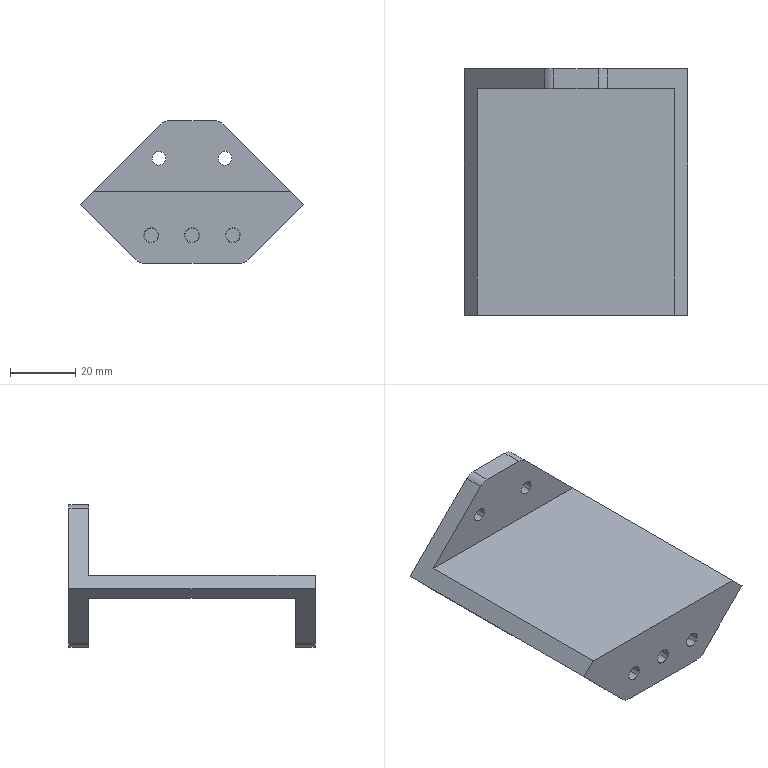Part | 1 solid | 42 faces | box 68.307 x 75.3 x 43.668 mm | volume 47119 mm3 | cylinder 20 | plane 16 | cone 6 | commonest cylinder face diameters 4.3 x6 8 x6 4 x4 4.2 x4
STEP:
#1=CARTESIAN_POINT('',(11.596,37.65,-13.01));
#2=VERTEX_POINT('',#1);
#3=CARTESIAN_POINT('',(8.626,37.65,-10.041));
#4=VERTEX_POINT('',#3);
#5=CARTESIAN_POINT('',(10.111,37.65,-11.525));
#6=DIRECTION('',(0.,-1.,0.));
#7=DIRECTION('',(-0.7071,0.,0.7071));
#8=AXIS2_PLACEMENT_3D('',#5,#6,#7);
#9=CIRCLE('',#8,2.1);
#10=EDGE_CURVE('',#2,#4,#9,.T.);
#11=ORIENTED_EDGE('',*,*,#10,.F.);
#12=CARTESIAN_POINT('',(11.596,31.65,-13.01));
#13=VERTEX_POINT('',#12);
#14=CARTESIAN_POINT('',(11.596,41.65,-13.01));
#15=DIRECTION('',(0.,-1.,0.));
#16=VECTOR('',#15,1000.);
#17=LINE('',#14,#16);
#18=EDGE_CURVE('',#13,#2,#17,.F.);
#19=ORIENTED_EDGE('',*,*,#18,.F.);
#20=CARTESIAN_POINT('',(8.626,31.65,-10.041));
#21=VERTEX_POINT('',#20);
#22=CARTESIAN_POINT('',(10.111,31.65,-11.525));
#23=DIRECTION('',(0.,-1.,0.));
#24=DIRECTION('',(-0.7071,0.,0.7071));
#25=AXIS2_PLACEMENT_3D('',#22,#23,#24);
#26=CIRCLE('',#25,2.1);
#27=EDGE_CURVE('',#13,#21,#26,.T.);
#28=ORIENTED_EDGE('',*,*,#27,.T.);
#29=CARTESIAN_POINT('',(8.626,41.65,-10.041));
#30=DIRECTION('',(0.,-1.,0.));
#31=VECTOR('',#30,1000.);
#32=LINE('',#29,#31);
#33=EDGE_CURVE('',#21,#4,#32,.F.);
#34=ORIENTED_EDGE('',*,*,#33,.T.);
#35=EDGE_LOOP('',(#11,#19,#28,#34));
#36=FACE_BOUND('',#35,.T.);
#37=CARTESIAN_POINT('',(10.111,41.65,-11.525));
#38=DIRECTION('',(0.,-1.,0.));
#39=DIRECTION('',(0.7071,0.,-0.7071));
#40=AXIS2_PLACEMENT_3D('',#37,#38,#39);
#41=CYLINDRICAL_SURFACE('',#40,2.1);
#42=ADVANCED_FACE('',(#36),#41,.F.);
#43=CARTESIAN_POINT('',(-8.626,37.65,-13.01));
#44=VERTEX_POINT('',#43);
#45=CARTESIAN_POINT('',(-11.596,37.65,-10.041));
#46=VERTEX_POINT('',#45);
#47=CARTESIAN_POINT('',(-10.111,37.65,-11.525));
#48=DIRECTION('',(0.,-1.,0.));
#49=DIRECTION('',(-0.7071,0.,0.7071));
#50=AXIS2_PLACEMENT_3D('',#47,#48,#49);
#51=CIRCLE('',#50,2.1);
#52=EDGE_CURVE('',#44,#46,#51,.T.);
#53=ORIENTED_EDGE('',*,*,#52,.F.);
#54=CARTESIAN_POINT('',(-8.626,31.65,-13.01));
#55=VERTEX_POINT('',#54);
#56=CARTESIAN_POINT('',(-8.626,41.65,-13.01));
#57=DIRECTION('',(0.,-1.,0.));
#58=VECTOR('',#57,1000.);
#59=LINE('',#56,#58);
#60=EDGE_CURVE('',#55,#44,#59,.F.);
#61=ORIENTED_EDGE('',*,*,#60,.F.);
#62=CARTESIAN_POINT('',(-11.596,31.65,-10.041));
#63=VERTEX_POINT('',#62);
#64=CARTESIAN_POINT('',(-10.111,31.65,-11.525));
#65=DIRECTION('',(0.,-1.,0.));
#66=DIRECTION('',(-0.7071,0.,0.7071));
#67=AXIS2_PLACEMENT_3D('',#64,#65,#66);
#68=CIRCLE('',#67,2.1);
#69=EDGE_CURVE('',#55,#63,#68,.T.);
#70=ORIENTED_EDGE('',*,*,#69,.T.);
#71=CARTESIAN_POINT('',(-11.596,41.65,-10.041));
#72=DIRECTION('',(0.,-1.,0.));
#73=VECTOR('',#72,1000.);
#74=LINE('',#71,#73);
#75=EDGE_CURVE('',#63,#46,#74,.F.);
#76=ORIENTED_EDGE('',*,*,#75,.T.);
#77=EDGE_LOOP('',(#53,#61,#70,#76));
#78=FACE_BOUND('',#77,.T.);
#79=CARTESIAN_POINT('',(-10.111,41.65,-11.525));
#80=DIRECTION('',(0.,-1.,0.));
#81=DIRECTION('',(0.7071,0.,-0.7071));
#82=AXIS2_PLACEMENT_3D('',#79,#80,#81);
#83=CYLINDRICAL_SURFACE('',#82,2.1);
#84=ADVANCED_FACE('',(#78),#83,.F.);
#85=CARTESIAN_POINT('',(3.536,33.65,-4.95));
#86=VERTEX_POINT('',#85);
#87=CARTESIAN_POINT('',(6.364,33.65,-7.778));
#88=VERTEX_POINT('',#87);
#89=CARTESIAN_POINT('',(4.95,33.65,-6.364));
#90=DIRECTION('',(0.,1.,0.));
#91=DIRECTION('',(0.7071,0.,-0.7071));
#92=AXIS2_PLACEMENT_3D('',#89,#90,#91);
#93=CIRCLE('',#92,2.);
#94=EDGE_CURVE('',#86,#88,#93,.T.);
#95=ORIENTED_EDGE('',*,*,#94,.F.);
#96=CARTESIAN_POINT('',(3.536,37.65,-4.95));
#97=VERTEX_POINT('',#96);
#98=CARTESIAN_POINT('',(3.536,33.65,-4.95));
#99=DIRECTION('',(0.,1.,0.));
#100=VECTOR('',#99,1000.);
#101=LINE('',#98,#100);
#102=EDGE_CURVE('',#97,#86,#101,.F.);
#103=ORIENTED_EDGE('',*,*,#102,.F.);
#104=CARTESIAN_POINT('',(6.364,37.65,-7.778));
#105=VERTEX_POINT('',#104);
#106=CARTESIAN_POINT('',(4.95,37.65,-6.364));
#107=DIRECTION('',(0.,1.,0.));
#108=DIRECTION('',(0.7071,0.,-0.7071));
#109=AXIS2_PLACEMENT_3D('',#106,#107,#108);
#110=CIRCLE('',#109,2.);
#111=EDGE_CURVE('',#97,#105,#110,.T.);
#112=ORIENTED_EDGE('',*,*,#111,.T.);
#113=CARTESIAN_POINT('',(6.364,33.65,-7.778));
#114=DIRECTION('',(0.,1.,0.));
#115=VECTOR('',#114,1000.);
#116=LINE('',#113,#115);
#117=EDGE_CURVE('',#105,#88,#116,.F.);
#118=ORIENTED_EDGE('',*,*,#117,.T.);
#119=EDGE_LOOP('',(#95,#103,#112,#118));
#120=FACE_BOUND('',#119,.T.);
#121=CARTESIAN_POINT('',(4.95,33.65,-6.364));
#122=DIRECTION('',(0.,1.,0.));
#123=DIRECTION('',(-0.7071,0.,0.7071));
#124=AXIS2_PLACEMENT_3D('',#121,#122,#123);
#125=CYLINDRICAL_SURFACE('',#124,2.);
#126=ADVANCED_FACE('',(#120),#125,.F.);
#127=CARTESIAN_POINT('',(-5.657,33.65,-14.142));
#128=VERTEX_POINT('',#127);
#129=CARTESIAN_POINT('',(-2.828,33.65,-16.971));
#130=VERTEX_POINT('',#129);
#131=CARTESIAN_POINT('',(-4.243,33.65,-15.556));
#132=DIRECTION('',(0.,1.,0.));
#133=DIRECTION('',(0.7071,0.,-0.7071));
#134=AXIS2_PLACEMENT_3D('',#131,#132,#133);
#135=CIRCLE('',#134,2.);
#136=EDGE_CURVE('',#128,#130,#135,.T.);
#137=ORIENTED_EDGE('',*,*,#136,.F.);
#138=CARTESIAN_POINT('',(-5.657,37.65,-14.142));
#139=VERTEX_POINT('',#138);
#140=CARTESIAN_POINT('',(-5.657,33.65,-14.142));
#141=DIRECTION('',(0.,1.,0.));
#142=VECTOR('',#141,1000.);
#143=LINE('',#140,#142);
#144=EDGE_CURVE('',#139,#128,#143,.F.);
#145=ORIENTED_EDGE('',*,*,#144,.F.);
#146=CARTESIAN_POINT('',(-2.828,37.65,-16.971));
#147=VERTEX_POINT('',#146);
#148=CARTESIAN_POINT('',(-4.243,37.65,-15.556));
#149=DIRECTION('',(0.,1.,0.));
#150=DIRECTION('',(0.7071,0.,-0.7071));
#151=AXIS2_PLACEMENT_3D('',#148,#149,#150);
#152=CIRCLE('',#151,2.);
#153=EDGE_CURVE('',#139,#147,#152,.T.);
#154=ORIENTED_EDGE('',*,*,#153,.T.);
#155=CARTESIAN_POINT('',(-2.828,33.65,-16.971));
#156=DIRECTION('',(0.,1.,0.));
#157=VECTOR('',#156,1000.);
#158=LINE('',#155,#157);
#159=EDGE_CURVE('',#147,#130,#158,.F.);
#160=ORIENTED_EDGE('',*,*,#159,.T.);
#161=EDGE_LOOP('',(#137,#145,#154,#160));
#162=FACE_BOUND('',#161,.T.);
#163=CARTESIAN_POINT('',(-4.243,33.65,-15.556));
#164=DIRECTION('',(0.,1.,0.));
#165=DIRECTION('',(-0.7071,0.,0.7071));
#166=AXIS2_PLACEMENT_3D('',#163,#164,#165);
#167=CYLINDRICAL_SURFACE('',#166,2.);
#168=ADVANCED_FACE('',(#162),#167,.F.);
#169=CARTESIAN_POINT('',(14.02,-37.525,-36.593));
#170=VERTEX_POINT('',#169);
#171=CARTESIAN_POINT('',(10.98,-37.525,-33.552));
#172=VERTEX_POINT('',#171);
#173=CARTESIAN_POINT('',(12.5,-37.525,-35.072));
#174=DIRECTION('',(0.,-1.,0.));
#175=DIRECTION('',(-0.7071,0.,0.7071));
#176=AXIS2_PLACEMENT_3D('',#173,#174,#175);
#177=CIRCLE('',#176,2.15);
#178=EDGE_CURVE('',#170,#172,#177,.T.);
#179=ORIENTED_EDGE('',*,*,#178,.F.);
#180=CARTESIAN_POINT('',(14.109,-37.65,-36.681));
#181=VERTEX_POINT('',#180);
#182=CARTESIAN_POINT('',(14.109,-37.65,-36.681));
#183=DIRECTION('',(0.5,-0.7071,-0.5));
#184=VECTOR('',#183,1000.);
#185=LINE('',#182,#184);
#186=EDGE_CURVE('',#181,#170,#185,.F.);
#187=ORIENTED_EDGE('',*,*,#186,.F.);
#188=CARTESIAN_POINT('',(10.891,-37.65,-33.464));
#189=VERTEX_POINT('',#188);
#190=CARTESIAN_POINT('',(12.5,-37.65,-35.072));
#191=DIRECTION('',(0.,-1.,0.));
#192=DIRECTION('',(-0.7071,0.,0.7071));
#193=AXIS2_PLACEMENT_3D('',#190,#191,#192);
#194=CIRCLE('',#193,2.275);
#195=EDGE_CURVE('',#181,#189,#194,.T.);
#196=ORIENTED_EDGE('',*,*,#195,.T.);
#197=CARTESIAN_POINT('',(10.891,-37.65,-33.464));
#198=DIRECTION('',(-0.5,-0.7071,0.5));
#199=VECTOR('',#198,1000.);
#200=LINE('',#197,#199);
#201=EDGE_CURVE('',#189,#172,#200,.F.);
#202=ORIENTED_EDGE('',*,*,#201,.T.);
#203=EDGE_LOOP('',(#179,#187,#196,#202));
#204=FACE_BOUND('',#203,.T.);
#205=CARTESIAN_POINT('',(12.5,-37.65,-35.072));
#206=DIRECTION('',(0.,-1.,0.));
#207=DIRECTION('',(0.7071,0.,-0.7071));
#208=AXIS2_PLACEMENT_3D('',#205,#206,#207);
#209=CONICAL_SURFACE('',#208,2.275,0.7854);
#210=ADVANCED_FACE('',(#204),#209,.F.);
#211=CARTESIAN_POINT('',(14.02,-31.65,-36.593));
#212=VERTEX_POINT('',#211);
#213=CARTESIAN_POINT('',(10.98,-31.65,-33.552));
#214=VERTEX_POINT('',#213);
#215=CARTESIAN_POINT('',(12.5,-31.65,-35.072));
#216=DIRECTION('',(0.,-1.,0.));
#217=DIRECTION('',(-0.7071,0.,0.7071));
#218=AXIS2_PLACEMENT_3D('',#215,#216,#217);
#219=CIRCLE('',#218,2.15);
#220=EDGE_CURVE('',#212,#214,#219,.T.);
#221=ORIENTED_EDGE('',*,*,#220,.F.);
#222=CARTESIAN_POINT('',(14.02,-37.65,-36.593));
#223=DIRECTION('',(0.,-1.,0.));
#224=VECTOR('',#223,1000.);
#225=LINE('',#222,#224);
#226=EDGE_CURVE('',#170,#212,#225,.F.);
#227=ORIENTED_EDGE('',*,*,#226,.F.);
#228=ORIENTED_EDGE('',*,*,#178,.T.);
#229=CARTESIAN_POINT('',(10.98,-37.65,-33.552));
#230=DIRECTION('',(0.,-1.,0.));
#231=VECTOR('',#230,1000.);
#232=LINE('',#229,#231);
#233=EDGE_CURVE('',#172,#214,#232,.F.);
#234=ORIENTED_EDGE('',*,*,#233,.T.);
#235=EDGE_LOOP('',(#221,#227,#228,#234));
#236=FACE_BOUND('',#235,.T.);
#237=CARTESIAN_POINT('',(12.5,-37.65,-35.072));
#238=DIRECTION('',(0.,-1.,0.));
#239=DIRECTION('',(0.7071,0.,-0.7071));
#240=AXIS2_PLACEMENT_3D('',#237,#238,#239);
#241=CYLINDRICAL_SURFACE('',#240,2.15);
#242=ADVANCED_FACE('',(#236),#241,.F.);
#243=CARTESIAN_POINT('',(1.52,-37.525,-36.593));
#244=VERTEX_POINT('',#243);
#245=CARTESIAN_POINT('',(-1.52,-37.525,-33.552));
#246=VERTEX_POINT('',#245);
#247=CARTESIAN_POINT('',(0.,-37.525,-35.072));
#248=DIRECTION('',(0.,-1.,0.));
#249=DIRECTION('',(-0.7071,0.,0.7071));
#250=AXIS2_PLACEMENT_3D('',#247,#248,#249);
#251=CIRCLE('',#250,2.15);
#252=EDGE_CURVE('',#244,#246,#251,.T.);
#253=ORIENTED_EDGE('',*,*,#252,.F.);
#254=CARTESIAN_POINT('',(1.609,-37.65,-36.681));
#255=VERTEX_POINT('',#254);
#256=CARTESIAN_POINT('',(1.609,-37.65,-36.681));
#257=DIRECTION('',(0.5,-0.7071,-0.5));
#258=VECTOR('',#257,1000.);
#259=LINE('',#256,#258);
#260=EDGE_CURVE('',#255,#244,#259,.F.);
#261=ORIENTED_EDGE('',*,*,#260,.F.);
#262=CARTESIAN_POINT('',(-1.609,-37.65,-33.464));
#263=VERTEX_POINT('',#262);
#264=CARTESIAN_POINT('',(0.,-37.65,-35.072));
#265=DIRECTION('',(0.,-1.,0.));
#266=DIRECTION('',(-0.7071,0.,0.7071));
#267=AXIS2_PLACEMENT_3D('',#264,#265,#266);
#268=CIRCLE('',#267,2.275);
#269=EDGE_CURVE('',#255,#263,#268,.T.);
#270=ORIENTED_EDGE('',*,*,#269,.T.);
#271=CARTESIAN_POINT('',(-1.609,-37.65,-33.464));
#272=DIRECTION('',(-0.5,-0.7071,0.5));
#273=VECTOR('',#272,1000.);
#274=LINE('',#271,#273);
#275=EDGE_CURVE('',#263,#246,#274,.F.);
#276=ORIENTED_EDGE('',*,*,#275,.T.);
#277=EDGE_LOOP('',(#253,#261,#270,#276));
#278=FACE_BOUND('',#277,.T.);
#279=CARTESIAN_POINT('',(0.,-37.65,-35.072));
#280=DIRECTION('',(0.,-1.,0.));
#281=DIRECTION('',(0.7071,0.,-0.7071));
#282=AXIS2_PLACEMENT_3D('',#279,#280,#281);
#283=CONICAL_SURFACE('',#282,2.275,0.7854);
#284=ADVANCED_FACE('',(#278),#283,.F.);
#285=CARTESIAN_POINT('',(1.52,-31.65,-36.593));
#286=VERTEX_POINT('',#285);
#287=CARTESIAN_POINT('',(-1.52,-31.65,-33.552));
#288=VERTEX_POINT('',#287);
#289=CARTESIAN_POINT('',(0.,-31.65,-35.072));
#290=DIRECTION('',(0.,-1.,0.));
#291=DIRECTION('',(-0.7071,0.,0.7071));
#292=AXIS2_PLACEMENT_3D('',#289,#290,#291);
#293=CIRCLE('',#292,2.15);
#294=EDGE_CURVE('',#286,#288,#293,.T.);
#295=ORIENTED_EDGE('',*,*,#294,.F.);
#296=CARTESIAN_POINT('',(1.52,-37.65,-36.593));
#297=DIRECTION('',(0.,-1.,0.));
#298=VECTOR('',#297,1000.);
#299=LINE('',#296,#298);
#300=EDGE_CURVE('',#244,#286,#299,.F.);
#301=ORIENTED_EDGE('',*,*,#300,.F.);
#302=ORIENTED_EDGE('',*,*,#252,.T.);
#303=CARTESIAN_POINT('',(-1.52,-37.65,-33.552));
#304=DIRECTION('',(0.,-1.,0.));
#305=VECTOR('',#304,1000.);
#306=LINE('',#303,#305);
#307=EDGE_CURVE('',#246,#288,#306,.F.);
#308=ORIENTED_EDGE('',*,*,#307,.T.);
#309=EDGE_LOOP('',(#295,#301,#302,#308));
#310=FACE_BOUND('',#309,.T.);
#311=CARTESIAN_POINT('',(0.,-37.65,-35.072));
#312=DIRECTION('',(0.,-1.,0.));
#313=DIRECTION('',(0.7071,0.,-0.7071));
#314=AXIS2_PLACEMENT_3D('',#311,#312,#313);
#315=CYLINDRICAL_SURFACE('',#314,2.15);
#316=ADVANCED_FACE('',(#310),#315,.F.);
#317=CARTESIAN_POINT('',(-10.98,-37.525,-36.593));
#318=VERTEX_POINT('',#317);
#319=CARTESIAN_POINT('',(-14.02,-37.525,-33.552));
#320=VERTEX_POINT('',#319);
#321=CARTESIAN_POINT('',(-12.5,-37.525,-35.072));
#322=DIRECTION('',(0.,-1.,0.));
#323=DIRECTION('',(-0.7071,0.,0.7071));
#324=AXIS2_PLACEMENT_3D('',#321,#322,#323);
#325=CIRCLE('',#324,2.15);
#326=EDGE_CURVE('',#318,#320,#325,.T.);
#327=ORIENTED_EDGE('',*,*,#326,.F.);
#328=CARTESIAN_POINT('',(-10.891,-37.65,-36.681));
#329=VERTEX_POINT('',#328);
#330=CARTESIAN_POINT('',(-10.891,-37.65,-36.681));
#331=DIRECTION('',(0.5,-0.7071,-0.5));
#332=VECTOR('',#331,1000.);
#333=LINE('',#330,#332);
#334=EDGE_CURVE('',#329,#318,#333,.F.);
#335=ORIENTED_EDGE('',*,*,#334,.F.);
#336=CARTESIAN_POINT('',(-14.109,-37.65,-33.464));
#337=VERTEX_POINT('',#336);
#338=CARTESIAN_POINT('',(-12.5,-37.65,-35.072));
#339=DIRECTION('',(0.,-1.,0.));
#340=DIRECTION('',(-0.7071,0.,0.7071));
#341=AXIS2_PLACEMENT_3D('',#338,#339,#340);
#342=CIRCLE('',#341,2.275);
#343=EDGE_CURVE('',#329,#337,#342,.T.);
#344=ORIENTED_EDGE('',*,*,#343,.T.);
#345=CARTESIAN_POINT('',(-14.109,-37.65,-33.464));
#346=DIRECTION('',(-0.5,-0.7071,0.5));
#347=VECTOR('',#346,1000.);
#348=LINE('',#345,#347);
#349=EDGE_CURVE('',#337,#320,#348,.F.);
#350=ORIENTED_EDGE('',*,*,#349,.T.);
#351=EDGE_LOOP('',(#327,#335,#344,#350));
#352=FACE_BOUND('',#351,.T.);
#353=CARTESIAN_POINT('',(-12.5,-37.65,-35.072));
#354=DIRECTION('',(0.,-1.,0.));
#355=DIRECTION('',(0.7071,0.,-0.7071));
#356=AXIS2_PLACEMENT_3D('',#353,#354,#355);
#357=CONICAL_SURFACE('',#356,2.275,0.7854);
#358=ADVANCED_FACE('',(#352),#357,.F.);
#359=CARTESIAN_POINT('',(-10.98,-31.65,-36.593));
#360=VERTEX_POINT('',#359);
#361=CARTESIAN_POINT('',(-14.02,-31.65,-33.552));
#362=VERTEX_POINT('',#361);
#363=CARTESIAN_POINT('',(-12.5,-31.65,-35.072));
#364=DIRECTION('',(0.,-1.,0.));
#365=DIRECTION('',(-0.7071,0.,0.7071));
#366=AXIS2_PLACEMENT_3D('',#363,#364,#365);
#367=CIRCLE('',#366,2.15);
#368=EDGE_CURVE('',#360,#362,#367,.T.);
#369=ORIENTED_EDGE('',*,*,#368,.F.);
#370=CARTESIAN_POINT('',(-10.98,-37.65,-36.593));
#371=DIRECTION('',(0.,-1.,0.));
#372=VECTOR('',#371,1000.);
#373=LINE('',#370,#372);
#374=EDGE_CURVE('',#318,#360,#373,.F.);
#375=ORIENTED_EDGE('',*,*,#374,.F.);
#376=ORIENTED_EDGE('',*,*,#326,.T.);
#377=CARTESIAN_POINT('',(-14.02,-37.65,-33.552));
#378=DIRECTION('',(0.,-1.,0.));
#379=VECTOR('',#378,1000.);
#380=LINE('',#377,#379);
#381=EDGE_CURVE('',#320,#362,#380,.F.);
#382=ORIENTED_EDGE('',*,*,#381,.T.);
#383=EDGE_LOOP('',(#369,#375,#376,#382));
#384=FACE_BOUND('',#383,.T.);
#385=CARTESIAN_POINT('',(-12.5,-37.65,-35.072));
#386=DIRECTION('',(0.,-1.,0.));
#387=DIRECTION('',(0.7071,0.,-0.7071));
#388=AXIS2_PLACEMENT_3D('',#385,#386,#387);
#389=CYLINDRICAL_SURFACE('',#388,2.15);
#390=ADVANCED_FACE('',(#384),#389,.F.);
#391=CARTESIAN_POINT('',(-31.153,31.65,-28.668));
#392=VERTEX_POINT('',#391);
#393=CARTESIAN_POINT('',(31.153,31.65,-28.668));
#394=VERTEX_POINT('',#393);
#395=CARTESIAN_POINT('',(-31.153,31.65,-28.668));
#396=DIRECTION('',(1.,0.,0.));
#397=VECTOR('',#396,1000.);
#398=LINE('',#395,#397);
#399=EDGE_CURVE('',#392,#394,#398,.T.);
#400=ORIENTED_EDGE('',*,*,#399,.T.);
#401=CARTESIAN_POINT('',(31.153,-31.65,-28.668));
#402=VERTEX_POINT('',#401);
#403=CARTESIAN_POINT('',(31.153,-99.957,-28.668));
#404=DIRECTION('',(0.,1.,0.));
#405=VECTOR('',#404,1000.);
#406=LINE('',#403,#405);
#407=EDGE_CURVE('',#402,#394,#406,.T.);
#408=ORIENTED_EDGE('',*,*,#407,.F.);
#409=CARTESIAN_POINT('',(-31.153,-31.65,-28.668));
#410=VERTEX_POINT('',#409);
#411=CARTESIAN_POINT('',(-31.153,-31.65,-28.668));
#412=DIRECTION('',(1.,0.,0.));
#413=VECTOR('',#412,1000.);
#414=LINE('',#411,#413);
#415=EDGE_CURVE('',#410,#402,#414,.T.);
#416=ORIENTED_EDGE('',*,*,#415,.F.);
#417=CARTESIAN_POINT('',(-31.153,-99.957,-28.668));
#418=DIRECTION('',(0.,1.,0.));
#419=VECTOR('',#418,1000.);
#420=LINE('',#417,#419);
#421=EDGE_CURVE('',#410,#392,#420,.T.);
#422=ORIENTED_EDGE('',*,*,#421,.T.);
#423=EDGE_LOOP('',(#400,#408,#416,#422));
#424=FACE_BOUND('',#423,.T.);
#425=CARTESIAN_POINT('',(-31.153,-99.957,-28.668));
#426=DIRECTION('',(0.,0.,1.));
#427=DIRECTION('',(1.,0.,0.));
#428=AXIS2_PLACEMENT_3D('',#425,#426,#427);
#429=PLANE('',#428);
#430=ADVANCED_FACE('',(#424),#429,.F.);
#431=CARTESIAN_POINT('',(-17.325,-31.65,-42.496));
#432=VERTEX_POINT('',#431);
#433=CARTESIAN_POINT('',(0.,-31.65,-59.821));
#434=DIRECTION('',(-0.7071,0.,0.7071));
#435=VECTOR('',#434,1000.);
#436=LINE('',#433,#435);
#437=EDGE_CURVE('',#432,#410,#436,.T.);
#438=ORIENTED_EDGE('',*,*,#437,.F.);
#439=CARTESIAN_POINT('',(-17.325,-37.65,-42.496));
#440=VERTEX_POINT('',#439);
#441=CARTESIAN_POINT('',(-17.325,-37.65,-42.496));
#442=DIRECTION('',(0.,-1.,0.));
#443=VECTOR('',#442,1000.);
#444=LINE('',#441,#443);
#445=EDGE_CURVE('',#432,#440,#444,.T.);
#446=ORIENTED_EDGE('',*,*,#445,.T.);
#447=CARTESIAN_POINT('',(-34.153,-37.65,-25.668));
#448=VERTEX_POINT('',#447);
#449=CARTESIAN_POINT('',(-16.153,-37.65,-43.668));
#450=DIRECTION('',(0.7071,0.,-0.7071));
#451=VECTOR('',#450,1000.);
#452=LINE('',#449,#451);
#453=EDGE_CURVE('',#448,#440,#452,.T.);
#454=ORIENTED_EDGE('',*,*,#453,.F.);
#455=CARTESIAN_POINT('',(-34.153,37.65,-25.668));
#456=VERTEX_POINT('',#455);
#457=CARTESIAN_POINT('',(-34.153,-37.65,-25.668));
#458=DIRECTION('',(0.,1.,0.));
#459=VECTOR('',#458,1000.);
#460=LINE('',#457,#459);
#461=EDGE_CURVE('',#448,#456,#460,.T.);
#462=ORIENTED_EDGE('',*,*,#461,.T.);
#463=CARTESIAN_POINT('',(-17.325,37.65,-42.496));
#464=VERTEX_POINT('',#463);
#465=CARTESIAN_POINT('',(-16.153,37.65,-43.668));
#466=DIRECTION('',(0.7071,0.,-0.7071));
#467=VECTOR('',#466,1000.);
#468=LINE('',#465,#467);
#469=EDGE_CURVE('',#456,#464,#468,.T.);
#470=ORIENTED_EDGE('',*,*,#469,.T.);
#471=CARTESIAN_POINT('',(-17.325,31.65,-42.496));
#472=VERTEX_POINT('',#471);
#473=CARTESIAN_POINT('',(-17.325,31.65,-42.496));
#474=DIRECTION('',(0.,1.,0.));
#475=VECTOR('',#474,1000.);
#476=LINE('',#473,#475);
#477=EDGE_CURVE('',#472,#464,#476,.T.);
#478=ORIENTED_EDGE('',*,*,#477,.F.);
#479=CARTESIAN_POINT('',(-17.325,31.65,-42.496));
#480=DIRECTION('',(-0.7071,0.,0.7071));
#481=VECTOR('',#480,1000.);
#482=LINE('',#479,#481);
#483=EDGE_CURVE('',#472,#392,#482,.T.);
#484=ORIENTED_EDGE('',*,*,#483,.T.);
#485=ORIENTED_EDGE('',*,*,#421,.F.);
#486=EDGE_LOOP('',(#438,#446,#454,#462,#470,#478,#484,#485));
#487=FACE_BOUND('',#486,.T.);
#488=CARTESIAN_POINT('',(-16.153,-37.65,-43.668));
#489=DIRECTION('',(0.7071,0.,0.7071));
#490=DIRECTION('',(0.7071,0.,-0.7071));
#491=AXIS2_PLACEMENT_3D('',#488,#489,#490);
#492=PLANE('',#491);
#493=ADVANCED_FACE('',(#487),#492,.F.);
#494=CARTESIAN_POINT('',(-14.496,-31.65,-43.668));
#495=VERTEX_POINT('',#494);
#496=CARTESIAN_POINT('',(14.496,-31.65,-43.668));
#497=VERTEX_POINT('',#496);
#498=CARTESIAN_POINT('',(16.153,-31.65,-43.668));
#499=DIRECTION('',(1.,0.,0.));
#500=VECTOR('',#499,1000.);
#501=LINE('',#498,#500);
#502=EDGE_CURVE('',#495,#497,#501,.T.);
#503=ORIENTED_EDGE('',*,*,#502,.T.);
#504=CARTESIAN_POINT('',(14.496,-37.65,-43.668));
#505=VERTEX_POINT('',#504);
#506=CARTESIAN_POINT('',(14.496,-37.65,-43.668));
#507=DIRECTION('',(0.,-1.,0.));
#508=VECTOR('',#507,1000.);
#509=LINE('',#506,#508);
#510=EDGE_CURVE('',#497,#505,#509,.T.);
#511=ORIENTED_EDGE('',*,*,#510,.T.);
#512=CARTESIAN_POINT('',(-14.496,-37.65,-43.668));
#513=VERTEX_POINT('',#512);
#514=CARTESIAN_POINT('',(16.153,-37.65,-43.668));
#515=DIRECTION('',(1.,0.,0.));
#516=VECTOR('',#515,1000.);
#517=LINE('',#514,#516);
#518=EDGE_CURVE('',#513,#505,#517,.T.);
#519=ORIENTED_EDGE('',*,*,#518,.F.);
#520=CARTESIAN_POINT('',(-14.496,-37.65,-43.668));
#521=DIRECTION('',(0.,1.,0.));
#522=VECTOR('',#521,1000.);
#523=LINE('',#520,#522);
#524=EDGE_CURVE('',#513,#495,#523,.T.);
#525=ORIENTED_EDGE('',*,*,#524,.T.);
#526=EDGE_LOOP('',(#503,#511,#519,#525));
#527=FACE_BOUND('',#526,.T.);
#528=CARTESIAN_POINT('',(16.153,-37.65,-43.668));
#529=DIRECTION('',(0.,0.,1.));
#530=DIRECTION('',(1.,0.,0.));
#531=AXIS2_PLACEMENT_3D('',#528,#529,#530);
#532=PLANE('',#531);
#533=ADVANCED_FACE('',(#527),#532,.F.);
#534=CARTESIAN_POINT('',(17.325,-37.65,-42.496));
#535=VERTEX_POINT('',#534);
#536=CARTESIAN_POINT('',(34.153,-37.65,-25.668));
#537=VERTEX_POINT('',#536);
#538=CARTESIAN_POINT('',(34.153,-37.65,-25.668));
#539=DIRECTION('',(0.7071,0.,0.7071));
#540=VECTOR('',#539,1000.);
#541=LINE('',#538,#540);
#542=EDGE_CURVE('',#535,#537,#541,.T.);
#543=ORIENTED_EDGE('',*,*,#542,.F.);
#544=CARTESIAN_POINT('',(17.325,-31.65,-42.496));
#545=VERTEX_POINT('',#544);
#546=CARTESIAN_POINT('',(17.325,-37.65,-42.496));
#547=DIRECTION('',(0.,1.,0.));
#548=VECTOR('',#547,1000.);
#549=LINE('',#546,#548);
#550=EDGE_CURVE('',#535,#545,#549,.T.);
#551=ORIENTED_EDGE('',*,*,#550,.T.);
#552=CARTESIAN_POINT('',(31.153,-31.65,-28.668));
#553=DIRECTION('',(-0.7071,0.,-0.7071));
#554=VECTOR('',#553,1000.);
#555=LINE('',#552,#554);
#556=EDGE_CURVE('',#402,#545,#555,.T.);
#557=ORIENTED_EDGE('',*,*,#556,.F.);
#558=ORIENTED_EDGE('',*,*,#407,.T.);
#559=CARTESIAN_POINT('',(17.325,31.65,-42.496));
#560=VERTEX_POINT('',#559);
#561=CARTESIAN_POINT('',(31.153,31.65,-28.668));
#562=DIRECTION('',(-0.7071,0.,-0.7071));
#563=VECTOR('',#562,1000.);
#564=LINE('',#561,#563);
#565=EDGE_CURVE('',#394,#560,#564,.T.);
#566=ORIENTED_EDGE('',*,*,#565,.T.);
#567=CARTESIAN_POINT('',(17.325,37.65,-42.496));
#568=VERTEX_POINT('',#567);
#569=CARTESIAN_POINT('',(17.325,31.65,-42.496));
#570=DIRECTION('',(0.,1.,0.));
#571=VECTOR('',#570,1000.);
#572=LINE('',#569,#571);
#573=EDGE_CURVE('',#560,#568,#572,.T.);
#574=ORIENTED_EDGE('',*,*,#573,.T.);
#575=CARTESIAN_POINT('',(34.153,37.65,-25.668));
#576=VERTEX_POINT('',#575);
#577=CARTESIAN_POINT('',(34.153,37.65,-25.668));
#578=DIRECTION('',(0.7071,0.,0.7071));
#579=VECTOR('',#578,1000.);
#580=LINE('',#577,#579);
#581=EDGE_CURVE('',#568,#576,#580,.T.);
#582=ORIENTED_EDGE('',*,*,#581,.T.);
#583=CARTESIAN_POINT('',(34.153,-37.65,-25.668));
#584=DIRECTION('',(0.,1.,0.));
#585=VECTOR('',#584,1000.);
#586=LINE('',#583,#585);
#587=EDGE_CURVE('',#537,#576,#586,.T.);
#588=ORIENTED_EDGE('',*,*,#587,.F.);
#589=EDGE_LOOP('',(#543,#551,#557,#558,#566,#574,#582,#588));
#590=FACE_BOUND('',#589,.T.);
#591=CARTESIAN_POINT('',(34.153,-37.65,-25.668));
#592=DIRECTION('',(-0.7071,0.,0.7071));
#593=DIRECTION('',(0.7071,0.,0.7071));
#594=AXIS2_PLACEMENT_3D('',#591,#592,#593);
#595=PLANE('',#594);
#596=ADVANCED_FACE('',(#590),#595,.F.);
#597=CARTESIAN_POINT('',(9.657,37.65,-1.172));
#598=VERTEX_POINT('',#597);
#599=CARTESIAN_POINT('',(34.153,37.65,-25.668));
#600=DIRECTION('',(-0.7071,0.,0.7071));
#601=VECTOR('',#600,1000.);
#602=LINE('',#599,#601);
#603=EDGE_CURVE('',#576,#598,#602,.T.);
#604=ORIENTED_EDGE('',*,*,#603,.T.);
#605=CARTESIAN_POINT('',(9.657,31.65,-1.172));
#606=VERTEX_POINT('',#605);
#607=CARTESIAN_POINT('',(9.657,-37.65,-1.172));
#608=DIRECTION('',(0.,-1.,0.));
#609=VECTOR('',#608,1000.);
#610=LINE('',#607,#609);
#611=EDGE_CURVE('',#598,#606,#610,.T.);
#612=ORIENTED_EDGE('',*,*,#611,.T.);
#613=CARTESIAN_POINT('',(30.153,31.65,-21.668));
#614=VERTEX_POINT('',#613);
#615=CARTESIAN_POINT('',(30.153,31.65,-21.668));
#616=DIRECTION('',(0.7071,0.,-0.7071));
#617=VECTOR('',#616,1000.);
#618=LINE('',#615,#617);
#619=EDGE_CURVE('',#606,#614,#618,.T.);
#620=ORIENTED_EDGE('',*,*,#619,.T.);
#621=CARTESIAN_POINT('',(30.153,-37.65,-21.668));
#622=VERTEX_POINT('',#621);
#623=CARTESIAN_POINT('',(30.153,97.957,-21.668));
#624=DIRECTION('',(0.,-1.,0.));
#625=VECTOR('',#624,1000.);
#626=LINE('',#623,#625);
#627=EDGE_CURVE('',#614,#622,#626,.T.);
#628=ORIENTED_EDGE('',*,*,#627,.T.);
#629=CARTESIAN_POINT('',(34.153,-37.65,-25.668));
#630=DIRECTION('',(-0.7071,0.,0.7071));
#631=VECTOR('',#630,1000.);
#632=LINE('',#629,#631);
#633=EDGE_CURVE('',#537,#622,#632,.T.);
#634=ORIENTED_EDGE('',*,*,#633,.F.);
#635=ORIENTED_EDGE('',*,*,#587,.T.);
#636=EDGE_LOOP('',(#604,#612,#620,#628,#634,#635));
#637=FACE_BOUND('',#636,.T.);
#638=CARTESIAN_POINT('',(34.153,-37.65,-25.668));
#639=DIRECTION('',(-0.7071,0.,-0.7071));
#640=DIRECTION('',(-0.7071,0.,0.7071));
#641=AXIS2_PLACEMENT_3D('',#638,#639,#640);
#642=PLANE('',#641);
#643=ADVANCED_FACE('',(#637),#642,.F.);
#644=CARTESIAN_POINT('',(-30.153,31.65,-21.668));
#645=VERTEX_POINT('',#644);
#646=CARTESIAN_POINT('',(-9.657,31.65,-1.172));
#647=VERTEX_POINT('',#646);
#648=CARTESIAN_POINT('',(0.,31.65,8.485));
#649=DIRECTION('',(0.7071,0.,0.7071));
#650=VECTOR('',#649,1000.);
#651=LINE('',#648,#650);
#652=EDGE_CURVE('',#645,#647,#651,.T.);
#653=ORIENTED_EDGE('',*,*,#652,.T.);
#654=CARTESIAN_POINT('',(-9.657,37.65,-1.172));
#655=VERTEX_POINT('',#654);
#656=CARTESIAN_POINT('',(-9.657,-37.65,-1.172));
#657=DIRECTION('',(0.,1.,0.));
#658=VECTOR('',#657,1000.);
#659=LINE('',#656,#658);
#660=EDGE_CURVE('',#647,#655,#659,.T.);
#661=ORIENTED_EDGE('',*,*,#660,.T.);
#662=CARTESIAN_POINT('',(0.,37.65,8.485));
#663=DIRECTION('',(-0.7071,0.,-0.7071));
#664=VECTOR('',#663,1000.);
#665=LINE('',#662,#664);
#666=EDGE_CURVE('',#655,#456,#665,.T.);
#667=ORIENTED_EDGE('',*,*,#666,.T.);
#668=ORIENTED_EDGE('',*,*,#461,.F.);
#669=CARTESIAN_POINT('',(-30.153,-37.65,-21.668));
#670=VERTEX_POINT('',#669);
#671=CARTESIAN_POINT('',(0.,-37.65,8.485));
#672=DIRECTION('',(-0.7071,0.,-0.7071));
#673=VECTOR('',#672,1000.);
#674=LINE('',#671,#673);
#675=EDGE_CURVE('',#670,#448,#674,.T.);
#676=ORIENTED_EDGE('',*,*,#675,.F.);
#677=CARTESIAN_POINT('',(-30.153,97.957,-21.668));
#678=DIRECTION('',(0.,-1.,0.));
#679=VECTOR('',#678,1000.);
#680=LINE('',#677,#679);
#681=EDGE_CURVE('',#645,#670,#680,.T.);
#682=ORIENTED_EDGE('',*,*,#681,.F.);
#683=EDGE_LOOP('',(#653,#661,#667,#668,#676,#682));
#684=FACE_BOUND('',#683,.T.);
#685=CARTESIAN_POINT('',(0.,-37.65,8.485));
#686=DIRECTION('',(0.7071,0.,-0.7071));
#687=DIRECTION('',(-0.7071,0.,-0.7071));
#688=AXIS2_PLACEMENT_3D('',#685,#686,#687);
#689=PLANE('',#688);
#690=ADVANCED_FACE('',(#684),#689,.F.);
#691=CARTESIAN_POINT('',(12.5,-37.65,-35.072));
#692=DIRECTION('',(0.,-1.,0.));
#693=DIRECTION('',(-0.7071,0.,0.7071));
#694=AXIS2_PLACEMENT_3D('',#691,#692,#693);
#695=CIRCLE('',#694,2.275);
#696=EDGE_CURVE('',#189,#181,#695,.T.);
#697=ORIENTED_EDGE('',*,*,#696,.F.);
#698=ORIENTED_EDGE('',*,*,#195,.F.);
#699=EDGE_LOOP('',(#697,#698));
#700=FACE_BOUND('',#699,.T.);
#701=CARTESIAN_POINT('',(0.,-37.65,-35.072));
#702=DIRECTION('',(0.,-1.,0.));
#703=DIRECTION('',(-0.7071,0.,0.7071));
#704=AXIS2_PLACEMENT_3D('',#701,#702,#703);
#705=CIRCLE('',#704,2.275);
#706=EDGE_CURVE('',#263,#255,#705,.T.);
#707=ORIENTED_EDGE('',*,*,#706,.F.);
#708=ORIENTED_EDGE('',*,*,#269,.F.);
#709=EDGE_LOOP('',(#707,#708));
#710=FACE_BOUND('',#709,.T.);
#711=CARTESIAN_POINT('',(-12.5,-37.65,-35.072));
#712=DIRECTION('',(0.,-1.,0.));
#713=DIRECTION('',(-0.7071,0.,0.7071));
#714=AXIS2_PLACEMENT_3D('',#711,#712,#713);
#715=CIRCLE('',#714,2.275);
#716=EDGE_CURVE('',#337,#329,#715,.T.);
#717=ORIENTED_EDGE('',*,*,#716,.F.);
#718=ORIENTED_EDGE('',*,*,#343,.F.);
#719=EDGE_LOOP('',(#717,#718));
#720=FACE_BOUND('',#719,.T.);
#721=ORIENTED_EDGE('',*,*,#518,.T.);
#722=CARTESIAN_POINT('',(14.496,-37.65,-39.668));
#723=DIRECTION('',(0.,-1.,0.));
#724=DIRECTION('',(-0.7071,0.,0.7071));
#725=AXIS2_PLACEMENT_3D('',#722,#723,#724);
#726=CIRCLE('',#725,4.);
#727=EDGE_CURVE('',#505,#535,#726,.T.);
#728=ORIENTED_EDGE('',*,*,#727,.T.);
#729=ORIENTED_EDGE('',*,*,#542,.T.);
#730=ORIENTED_EDGE('',*,*,#633,.T.);
#731=CARTESIAN_POINT('',(-30.153,-37.65,-21.668));
#732=DIRECTION('',(1.,0.,0.));
#733=VECTOR('',#732,1000.);
#734=LINE('',#731,#733);
#735=EDGE_CURVE('',#670,#622,#734,.T.);
#736=ORIENTED_EDGE('',*,*,#735,.F.);
#737=ORIENTED_EDGE('',*,*,#675,.T.);
#738=ORIENTED_EDGE('',*,*,#453,.T.);
#739=CARTESIAN_POINT('',(-14.496,-37.65,-39.668));
#740=DIRECTION('',(0.,-1.,0.));
#741=DIRECTION('',(-0.7071,0.,0.7071));
#742=AXIS2_PLACEMENT_3D('',#739,#740,#741);
#743=CIRCLE('',#742,4.);
#744=EDGE_CURVE('',#440,#513,#743,.T.);
#745=ORIENTED_EDGE('',*,*,#744,.T.);
#746=EDGE_LOOP('',(#721,#728,#729,#730,#736,#737,#738,#745));
#747=FACE_BOUND('',#746,.T.);
#748=CARTESIAN_POINT('',(0.,-37.65,-25.668));
#749=DIRECTION('',(0.,-1.,0.));
#750=DIRECTION('',(0.7071,0.,-0.7071));
#751=AXIS2_PLACEMENT_3D('',#748,#749,#750);
#752=PLANE('',#751);
#753=ADVANCED_FACE('',(#700,#710,#720,#747),#752,.T.);
#754=CARTESIAN_POINT('',(10.111,37.65,-11.525));
#755=DIRECTION('',(0.,-1.,0.));
#756=DIRECTION('',(-0.7071,0.,0.7071));
#757=AXIS2_PLACEMENT_3D('',#754,#755,#756);
#758=CIRCLE('',#757,2.1);
#759=EDGE_CURVE('',#4,#2,#758,.T.);
#760=ORIENTED_EDGE('',*,*,#759,.T.);
#761=ORIENTED_EDGE('',*,*,#10,.T.);
#762=EDGE_LOOP('',(#760,#761));
#763=FACE_BOUND('',#762,.T.);
#764=CARTESIAN_POINT('',(-10.111,37.65,-11.525));
#765=DIRECTION('',(0.,-1.,0.));
#766=DIRECTION('',(-0.7071,0.,0.7071));
#767=AXIS2_PLACEMENT_3D('',#764,#765,#766);
#768=CIRCLE('',#767,2.1);
#769=EDGE_CURVE('',#46,#44,#768,.T.);
#770=ORIENTED_EDGE('',*,*,#769,.T.);
#771=ORIENTED_EDGE('',*,*,#52,.T.);
#772=EDGE_LOOP('',(#770,#771));
#773=FACE_BOUND('',#772,.T.);
#774=CARTESIAN_POINT('',(4.95,37.65,-6.364));
#775=DIRECTION('',(0.,1.,0.));
#776=DIRECTION('',(0.7071,0.,-0.7071));
#777=AXIS2_PLACEMENT_3D('',#774,#775,#776);
#778=CIRCLE('',#777,2.);
#779=EDGE_CURVE('',#105,#97,#778,.T.);
#780=ORIENTED_EDGE('',*,*,#779,.F.);
#781=ORIENTED_EDGE('',*,*,#111,.F.);
#782=EDGE_LOOP('',(#780,#781));
#783=FACE_BOUND('',#782,.T.);
#784=CARTESIAN_POINT('',(-4.243,37.65,-15.556));
#785=DIRECTION('',(0.,1.,0.));
#786=DIRECTION('',(0.7071,0.,-0.7071));
#787=AXIS2_PLACEMENT_3D('',#784,#785,#786);
#788=CIRCLE('',#787,2.);
#789=EDGE_CURVE('',#147,#139,#788,.T.);
#790=ORIENTED_EDGE('',*,*,#789,.F.);
#791=ORIENTED_EDGE('',*,*,#153,.F.);
#792=EDGE_LOOP('',(#790,#791));
#793=FACE_BOUND('',#792,.T.);
#794=ORIENTED_EDGE('',*,*,#666,.F.);
#795=CARTESIAN_POINT('',(-6.828,37.65,0.));
#796=VERTEX_POINT('',#795);
#797=CARTESIAN_POINT('',(-6.828,37.65,-4.));
#798=DIRECTION('',(0.,1.,0.));
#799=DIRECTION('',(-0.7071,0.,0.7071));
#800=AXIS2_PLACEMENT_3D('',#797,#798,#799);
#801=CIRCLE('',#800,4.);
#802=EDGE_CURVE('',#655,#796,#801,.T.);
#803=ORIENTED_EDGE('',*,*,#802,.T.);
#804=CARTESIAN_POINT('',(6.828,37.65,0.));
#805=VERTEX_POINT('',#804);
#806=CARTESIAN_POINT('',(8.485,37.65,0.));
#807=DIRECTION('',(-1.,0.,0.));
#808=VECTOR('',#807,1000.);
#809=LINE('',#806,#808);
#810=EDGE_CURVE('',#805,#796,#809,.T.);
#811=ORIENTED_EDGE('',*,*,#810,.F.);
#812=CARTESIAN_POINT('',(6.828,37.65,-4.));
#813=DIRECTION('',(0.,1.,0.));
#814=DIRECTION('',(-0.7071,0.,0.7071));
#815=AXIS2_PLACEMENT_3D('',#812,#813,#814);
#816=CIRCLE('',#815,4.);
#817=EDGE_CURVE('',#805,#598,#816,.T.);
#818=ORIENTED_EDGE('',*,*,#817,.T.);
#819=ORIENTED_EDGE('',*,*,#603,.F.);
#820=ORIENTED_EDGE('',*,*,#581,.F.);
#821=CARTESIAN_POINT('',(14.496,37.65,-43.668));
#822=VERTEX_POINT('',#821);
#823=CARTESIAN_POINT('',(14.496,37.65,-39.668));
#824=DIRECTION('',(0.,1.,0.));
#825=DIRECTION('',(0.7071,0.,-0.7071));
#826=AXIS2_PLACEMENT_3D('',#823,#824,#825);
#827=CIRCLE('',#826,4.);
#828=EDGE_CURVE('',#568,#822,#827,.T.);
#829=ORIENTED_EDGE('',*,*,#828,.T.);
#830=CARTESIAN_POINT('',(-14.496,37.65,-43.668));
#831=VERTEX_POINT('',#830);
#832=CARTESIAN_POINT('',(-14.496,37.65,-43.668));
#833=DIRECTION('',(-1.,0.,0.));
#834=VECTOR('',#833,1000.);
#835=LINE('',#832,#834);
#836=EDGE_CURVE('',#822,#831,#835,.T.);
#837=ORIENTED_EDGE('',*,*,#836,.T.);
#838=CARTESIAN_POINT('',(-14.496,37.65,-39.668));
#839=DIRECTION('',(0.,1.,0.));
#840=DIRECTION('',(0.7071,0.,-0.7071));
#841=AXIS2_PLACEMENT_3D('',#838,#839,#840);
#842=CIRCLE('',#841,4.);
#843=EDGE_CURVE('',#831,#464,#842,.T.);
#844=ORIENTED_EDGE('',*,*,#843,.T.);
#845=ORIENTED_EDGE('',*,*,#469,.F.);
#846=EDGE_LOOP('',(#794,#803,#811,#818,#819,#820,#829,#837,#844,#845));
#847=FACE_BOUND('',#846,.T.);
#848=CARTESIAN_POINT('',(0.,37.65,-25.668));
#849=DIRECTION('',(0.,-1.,0.));
#850=DIRECTION('',(0.7071,0.,-0.7071));
#851=AXIS2_PLACEMENT_3D('',#848,#849,#850);
#852=PLANE('',#851);
#853=ADVANCED_FACE('',(#763,#773,#783,#793,#847),#852,.F.);
#854=CARTESIAN_POINT('',(-30.153,31.65,-21.668));
#855=DIRECTION('',(-1.,0.,0.));
#856=VECTOR('',#855,1000.);
#857=LINE('',#854,#856);
#858=EDGE_CURVE('',#614,#645,#857,.T.);
#859=ORIENTED_EDGE('',*,*,#858,.T.);
#860=ORIENTED_EDGE('',*,*,#681,.T.);
#861=ORIENTED_EDGE('',*,*,#735,.T.);
#862=ORIENTED_EDGE('',*,*,#627,.F.);
#863=EDGE_LOOP('',(#859,#860,#861,#862));
#864=FACE_BOUND('',#863,.T.);
#865=CARTESIAN_POINT('',(-30.153,97.957,-21.668));
#866=DIRECTION('',(0.,0.,-1.));
#867=DIRECTION('',(-1.,0.,0.));
#868=AXIS2_PLACEMENT_3D('',#865,#866,#867);
#869=PLANE('',#868);
#870=ADVANCED_FACE('',(#864),#869,.F.);
#871=CARTESIAN_POINT('',(10.111,31.65,-11.525));
#872=DIRECTION('',(0.,-1.,0.));
#873=DIRECTION('',(-0.7071,0.,0.7071));
#874=AXIS2_PLACEMENT_3D('',#871,#872,#873);
#875=CIRCLE('',#874,2.1);
#876=EDGE_CURVE('',#21,#13,#875,.T.);
#877=ORIENTED_EDGE('',*,*,#876,.F.);
#878=ORIENTED_EDGE('',*,*,#27,.F.);
#879=EDGE_LOOP('',(#877,#878));
#880=FACE_BOUND('',#879,.T.);
#881=CARTESIAN_POINT('',(-10.111,31.65,-11.525));
#882=DIRECTION('',(0.,-1.,0.));
#883=DIRECTION('',(-0.7071,0.,0.7071));
#884=AXIS2_PLACEMENT_3D('',#881,#882,#883);
#885=CIRCLE('',#884,2.1);
#886=EDGE_CURVE('',#63,#55,#885,.T.);
#887=ORIENTED_EDGE('',*,*,#886,.F.);
#888=ORIENTED_EDGE('',*,*,#69,.F.);
#889=EDGE_LOOP('',(#887,#888));
#890=FACE_BOUND('',#889,.T.);
#891=CARTESIAN_POINT('',(-6.828,31.65,0.));
#892=VERTEX_POINT('',#891);
#893=CARTESIAN_POINT('',(6.828,31.65,0.));
#894=VERTEX_POINT('',#893);
#895=CARTESIAN_POINT('',(0.,31.65,0.));
#896=DIRECTION('',(1.,0.,0.));
#897=VECTOR('',#896,1000.);
#898=LINE('',#895,#897);
#899=EDGE_CURVE('',#892,#894,#898,.T.);
#900=ORIENTED_EDGE('',*,*,#899,.F.);
#901=CARTESIAN_POINT('',(-6.828,31.65,-4.));
#902=DIRECTION('',(0.,-1.,0.));
#903=DIRECTION('',(-0.7071,0.,0.7071));
#904=AXIS2_PLACEMENT_3D('',#901,#902,#903);
#905=CIRCLE('',#904,4.);
#906=EDGE_CURVE('',#892,#647,#905,.T.);
#907=ORIENTED_EDGE('',*,*,#906,.T.);
#908=ORIENTED_EDGE('',*,*,#652,.F.);
#909=ORIENTED_EDGE('',*,*,#858,.F.);
#910=ORIENTED_EDGE('',*,*,#619,.F.);
#911=CARTESIAN_POINT('',(6.828,31.65,-4.));
#912=DIRECTION('',(0.,-1.,0.));
#913=DIRECTION('',(-0.7071,0.,0.7071));
#914=AXIS2_PLACEMENT_3D('',#911,#912,#913);
#915=CIRCLE('',#914,4.);
#916=EDGE_CURVE('',#606,#894,#915,.T.);
#917=ORIENTED_EDGE('',*,*,#916,.T.);
#918=EDGE_LOOP('',(#900,#907,#908,#909,#910,#917));
#919=FACE_BOUND('',#918,.T.);
#920=CARTESIAN_POINT('',(0.,31.65,-25.668));
#921=DIRECTION('',(0.,-1.,0.));
#922=DIRECTION('',(0.7071,0.,-0.7071));
#923=AXIS2_PLACEMENT_3D('',#920,#921,#922);
#924=PLANE('',#923);
#925=ADVANCED_FACE('',(#880,#890,#919),#924,.T.);
#926=CARTESIAN_POINT('',(12.5,-31.65,-35.072));
#927=DIRECTION('',(0.,-1.,0.));
#928=DIRECTION('',(-0.7071,0.,0.7071));
#929=AXIS2_PLACEMENT_3D('',#926,#927,#928);
#930=CIRCLE('',#929,2.15);
#931=EDGE_CURVE('',#214,#212,#930,.T.);
#932=ORIENTED_EDGE('',*,*,#931,.T.);
#933=ORIENTED_EDGE('',*,*,#220,.T.);
#934=EDGE_LOOP('',(#932,#933));
#935=FACE_BOUND('',#934,.T.);
#936=CARTESIAN_POINT('',(0.,-31.65,-35.072));
#937=DIRECTION('',(0.,-1.,0.));
#938=DIRECTION('',(-0.7071,0.,0.7071));
#939=AXIS2_PLACEMENT_3D('',#936,#937,#938);
#940=CIRCLE('',#939,2.15);
#941=EDGE_CURVE('',#288,#286,#940,.T.);
#942=ORIENTED_EDGE('',*,*,#941,.T.);
#943=ORIENTED_EDGE('',*,*,#294,.T.);
#944=EDGE_LOOP('',(#942,#943));
#945=FACE_BOUND('',#944,.T.);
#946=CARTESIAN_POINT('',(-12.5,-31.65,-35.072));
#947=DIRECTION('',(0.,-1.,0.));
#948=DIRECTION('',(-0.7071,0.,0.7071));
#949=AXIS2_PLACEMENT_3D('',#946,#947,#948);
#950=CIRCLE('',#949,2.15);
#951=EDGE_CURVE('',#362,#360,#950,.T.);
#952=ORIENTED_EDGE('',*,*,#951,.T.);
#953=ORIENTED_EDGE('',*,*,#368,.T.);
#954=EDGE_LOOP('',(#952,#953));
#955=FACE_BOUND('',#954,.T.);
#956=ORIENTED_EDGE('',*,*,#556,.T.);
#957=CARTESIAN_POINT('',(14.496,-31.65,-39.668));
#958=DIRECTION('',(0.,1.,0.));
#959=DIRECTION('',(-0.7071,0.,0.7071));
#960=AXIS2_PLACEMENT_3D('',#957,#958,#959);
#961=CIRCLE('',#960,4.);
#962=EDGE_CURVE('',#545,#497,#961,.T.);
#963=ORIENTED_EDGE('',*,*,#962,.T.);
#964=ORIENTED_EDGE('',*,*,#502,.F.);
#965=CARTESIAN_POINT('',(-14.496,-31.65,-39.668));
#966=DIRECTION('',(0.,1.,0.));
#967=DIRECTION('',(-0.7071,0.,0.7071));
#968=AXIS2_PLACEMENT_3D('',#965,#966,#967);
#969=CIRCLE('',#968,4.);
#970=EDGE_CURVE('',#495,#432,#969,.T.);
#971=ORIENTED_EDGE('',*,*,#970,.T.);
#972=ORIENTED_EDGE('',*,*,#437,.T.);
#973=ORIENTED_EDGE('',*,*,#415,.T.);
#974=EDGE_LOOP('',(#956,#963,#964,#971,#972,#973));
#975=FACE_BOUND('',#974,.T.);
#976=CARTESIAN_POINT('',(0.,-31.65,-25.668));
#977=DIRECTION('',(0.,-1.,0.));
#978=DIRECTION('',(0.7071,0.,-0.7071));
#979=AXIS2_PLACEMENT_3D('',#976,#977,#978);
#980=PLANE('',#979);
#981=ADVANCED_FACE('',(#935,#945,#955,#975),#980,.F.);
#982=ORIENTED_EDGE('',*,*,#374,.T.);
#983=ORIENTED_EDGE('',*,*,#951,.F.);
#984=ORIENTED_EDGE('',*,*,#381,.F.);
#985=CARTESIAN_POINT('',(-12.5,-37.525,-35.072));
#986=DIRECTION('',(0.,-1.,0.));
#987=DIRECTION('',(-0.7071,0.,0.7071));
#988=AXIS2_PLACEMENT_3D('',#985,#986,#987);
#989=CIRCLE('',#988,2.15);
#990=EDGE_CURVE('',#320,#318,#989,.T.);
#991=ORIENTED_EDGE('',*,*,#990,.T.);
#992=EDGE_LOOP('',(#982,#983,#984,#991));
#993=FACE_BOUND('',#992,.T.);
#994=CARTESIAN_POINT('',(-12.5,-37.65,-35.072));
#995=DIRECTION('',(0.,-1.,0.));
#996=DIRECTION('',(0.7071,0.,-0.7071));
#997=AXIS2_PLACEMENT_3D('',#994,#995,#996);
#998=CYLINDRICAL_SURFACE('',#997,2.15);
#999=ADVANCED_FACE('',(#993),#998,.F.);
#1000=ORIENTED_EDGE('',*,*,#334,.T.);
#1001=ORIENTED_EDGE('',*,*,#990,.F.);
#1002=ORIENTED_EDGE('',*,*,#349,.F.);
#1003=ORIENTED_EDGE('',*,*,#716,.T.);
#1004=EDGE_LOOP('',(#1000,#1001,#1002,#1003));
#1005=FACE_BOUND('',#1004,.T.);
#1006=CARTESIAN_POINT('',(-12.5,-37.65,-35.072));
#1007=DIRECTION('',(0.,-1.,0.));
#1008=DIRECTION('',(0.7071,0.,-0.7071));
#1009=AXIS2_PLACEMENT_3D('',#1006,#1007,#1008);
#1010=CONICAL_SURFACE('',#1009,2.275,0.7854);
#1011=ADVANCED_FACE('',(#1005),#1010,.F.);
#1012=ORIENTED_EDGE('',*,*,#300,.T.);
#1013=ORIENTED_EDGE('',*,*,#941,.F.);
#1014=ORIENTED_EDGE('',*,*,#307,.F.);
#1015=CARTESIAN_POINT('',(0.,-37.525,-35.072));
#1016=DIRECTION('',(0.,-1.,0.));
#1017=DIRECTION('',(-0.7071,0.,0.7071));
#1018=AXIS2_PLACEMENT_3D('',#1015,#1016,#1017);
#1019=CIRCLE('',#1018,2.15);
#1020=EDGE_CURVE('',#246,#244,#1019,.T.);
#1021=ORIENTED_EDGE('',*,*,#1020,.T.);
#1022=EDGE_LOOP('',(#1012,#1013,#1014,#1021));
#1023=FACE_BOUND('',#1022,.T.);
#1024=CARTESIAN_POINT('',(0.,-37.65,-35.072));
#1025=DIRECTION('',(0.,-1.,0.));
#1026=DIRECTION('',(0.7071,0.,-0.7071));
#1027=AXIS2_PLACEMENT_3D('',#1024,#1025,#1026);
#1028=CYLINDRICAL_SURFACE('',#1027,2.15);
#1029=ADVANCED_FACE('',(#1023),#1028,.F.);
#1030=ORIENTED_EDGE('',*,*,#260,.T.);
#1031=ORIENTED_EDGE('',*,*,#1020,.F.);
#1032=ORIENTED_EDGE('',*,*,#275,.F.);
#1033=ORIENTED_EDGE('',*,*,#706,.T.);
#1034=EDGE_LOOP('',(#1030,#1031,#1032,#1033));
#1035=FACE_BOUND('',#1034,.T.);
#1036=CARTESIAN_POINT('',(0.,-37.65,-35.072));
#1037=DIRECTION('',(0.,-1.,0.));
#1038=DIRECTION('',(0.7071,0.,-0.7071));
#1039=AXIS2_PLACEMENT_3D('',#1036,#1037,#1038);
#1040=CONICAL_SURFACE('',#1039,2.275,0.7854);
#1041=ADVANCED_FACE('',(#1035),#1040,.F.);
#1042=ORIENTED_EDGE('',*,*,#226,.T.);
#1043=ORIENTED_EDGE('',*,*,#931,.F.);
#1044=ORIENTED_EDGE('',*,*,#233,.F.);
#1045=CARTESIAN_POINT('',(12.5,-37.525,-35.072));
#1046=DIRECTION('',(0.,-1.,0.));
#1047=DIRECTION('',(-0.7071,0.,0.7071));
#1048=AXIS2_PLACEMENT_3D('',#1045,#1046,#1047);
#1049=CIRCLE('',#1048,2.15);
#1050=EDGE_CURVE('',#172,#170,#1049,.T.);
#1051=ORIENTED_EDGE('',*,*,#1050,.T.);
#1052=EDGE_LOOP('',(#1042,#1043,#1044,#1051));
#1053=FACE_BOUND('',#1052,.T.);
#1054=CARTESIAN_POINT('',(12.5,-37.65,-35.072));
#1055=DIRECTION('',(0.,-1.,0.));
#1056=DIRECTION('',(0.7071,0.,-0.7071));
#1057=AXIS2_PLACEMENT_3D('',#1054,#1055,#1056);
#1058=CYLINDRICAL_SURFACE('',#1057,2.15);
#1059=ADVANCED_FACE('',(#1053),#1058,.F.);
#1060=ORIENTED_EDGE('',*,*,#186,.T.);
#1061=ORIENTED_EDGE('',*,*,#1050,.F.);
#1062=ORIENTED_EDGE('',*,*,#201,.F.);
#1063=ORIENTED_EDGE('',*,*,#696,.T.);
#1064=EDGE_LOOP('',(#1060,#1061,#1062,#1063));
#1065=FACE_BOUND('',#1064,.T.);
#1066=CARTESIAN_POINT('',(12.5,-37.65,-35.072));
#1067=DIRECTION('',(0.,-1.,0.));
#1068=DIRECTION('',(0.7071,0.,-0.7071));
#1069=AXIS2_PLACEMENT_3D('',#1066,#1067,#1068);
#1070=CONICAL_SURFACE('',#1069,2.275,0.7854);
#1071=ADVANCED_FACE('',(#1065),#1070,.F.);
#1072=ORIENTED_EDGE('',*,*,#727,.F.);
#1073=ORIENTED_EDGE('',*,*,#510,.F.);
#1074=ORIENTED_EDGE('',*,*,#962,.F.);
#1075=ORIENTED_EDGE('',*,*,#550,.F.);
#1076=EDGE_LOOP('',(#1072,#1073,#1074,#1075));
#1077=FACE_BOUND('',#1076,.T.);
#1078=CARTESIAN_POINT('',(14.496,-37.65,-39.668));
#1079=DIRECTION('',(0.,1.,0.));
#1080=DIRECTION('',(-0.7071,0.,0.7071));
#1081=AXIS2_PLACEMENT_3D('',#1078,#1079,#1080);
#1082=CYLINDRICAL_SURFACE('',#1081,4.);
#1083=ADVANCED_FACE('',(#1077),#1082,.T.);
#1084=ORIENTED_EDGE('',*,*,#744,.F.);
#1085=ORIENTED_EDGE('',*,*,#445,.F.);
#1086=ORIENTED_EDGE('',*,*,#970,.F.);
#1087=ORIENTED_EDGE('',*,*,#524,.F.);
#1088=EDGE_LOOP('',(#1084,#1085,#1086,#1087));
#1089=FACE_BOUND('',#1088,.T.);
#1090=CARTESIAN_POINT('',(-14.496,-37.65,-39.668));
#1091=DIRECTION('',(0.,1.,0.));
#1092=DIRECTION('',(-0.7071,0.,0.7071));
#1093=AXIS2_PLACEMENT_3D('',#1090,#1091,#1092);
#1094=CYLINDRICAL_SURFACE('',#1093,4.);
#1095=ADVANCED_FACE('',(#1089),#1094,.T.);
#1096=ORIENTED_EDGE('',*,*,#144,.T.);
#1097=CARTESIAN_POINT('',(-4.243,33.65,-15.556));
#1098=DIRECTION('',(0.,1.,0.));
#1099=DIRECTION('',(0.7071,0.,-0.7071));
#1100=AXIS2_PLACEMENT_3D('',#1097,#1098,#1099);
#1101=CIRCLE('',#1100,2.);
#1102=EDGE_CURVE('',#130,#128,#1101,.T.);
#1103=ORIENTED_EDGE('',*,*,#1102,.F.);
#1104=ORIENTED_EDGE('',*,*,#159,.F.);
#1105=ORIENTED_EDGE('',*,*,#789,.T.);
#1106=EDGE_LOOP('',(#1096,#1103,#1104,#1105));
#1107=FACE_BOUND('',#1106,.T.);
#1108=CARTESIAN_POINT('',(-4.243,33.65,-15.556));
#1109=DIRECTION('',(0.,1.,0.));
#1110=DIRECTION('',(-0.7071,0.,0.7071));
#1111=AXIS2_PLACEMENT_3D('',#1108,#1109,#1110);
#1112=CYLINDRICAL_SURFACE('',#1111,2.);
#1113=ADVANCED_FACE('',(#1107),#1112,.F.);
#1114=ORIENTED_EDGE('',*,*,#1102,.T.);
#1115=ORIENTED_EDGE('',*,*,#136,.T.);
#1116=EDGE_LOOP('',(#1114,#1115));
#1117=FACE_BOUND('',#1116,.T.);
#1118=CARTESIAN_POINT('',(-4.243,33.65,-15.556));
#1119=DIRECTION('',(0.,1.,0.));
#1120=DIRECTION('',(-0.7071,0.,0.7071));
#1121=AXIS2_PLACEMENT_3D('',#1118,#1119,#1120);
#1122=PLANE('',#1121);
#1123=ADVANCED_FACE('',(#1117),#1122,.T.);
#1124=ORIENTED_EDGE('',*,*,#102,.T.);
#1125=CARTESIAN_POINT('',(4.95,33.65,-6.364));
#1126=DIRECTION('',(0.,1.,0.));
#1127=DIRECTION('',(0.7071,0.,-0.7071));
#1128=AXIS2_PLACEMENT_3D('',#1125,#1126,#1127);
#1129=CIRCLE('',#1128,2.);
#1130=EDGE_CURVE('',#88,#86,#1129,.T.);
#1131=ORIENTED_EDGE('',*,*,#1130,.F.);
#1132=ORIENTED_EDGE('',*,*,#117,.F.);
#1133=ORIENTED_EDGE('',*,*,#779,.T.);
#1134=EDGE_LOOP('',(#1124,#1131,#1132,#1133));
#1135=FACE_BOUND('',#1134,.T.);
#1136=CARTESIAN_POINT('',(4.95,33.65,-6.364));
#1137=DIRECTION('',(0.,1.,0.));
#1138=DIRECTION('',(-0.7071,0.,0.7071));
#1139=AXIS2_PLACEMENT_3D('',#1136,#1137,#1138);
#1140=CYLINDRICAL_SURFACE('',#1139,2.);
#1141=ADVANCED_FACE('',(#1135),#1140,.F.);
#1142=ORIENTED_EDGE('',*,*,#1130,.T.);
#1143=ORIENTED_EDGE('',*,*,#94,.T.);
#1144=EDGE_LOOP('',(#1142,#1143));
#1145=FACE_BOUND('',#1144,.T.);
#1146=CARTESIAN_POINT('',(4.95,33.65,-6.364));
#1147=DIRECTION('',(0.,1.,0.));
#1148=DIRECTION('',(-0.7071,0.,0.7071));
#1149=AXIS2_PLACEMENT_3D('',#1146,#1147,#1148);
#1150=PLANE('',#1149);
#1151=ADVANCED_FACE('',(#1145),#1150,.T.);
#1152=ORIENTED_EDGE('',*,*,#810,.T.);
#1153=CARTESIAN_POINT('',(-6.828,-37.65,0.));
#1154=DIRECTION('',(0.,-1.,0.));
#1155=VECTOR('',#1154,1000.);
#1156=LINE('',#1153,#1155);
#1157=EDGE_CURVE('',#796,#892,#1156,.T.);
#1158=ORIENTED_EDGE('',*,*,#1157,.T.);
#1159=ORIENTED_EDGE('',*,*,#899,.T.);
#1160=CARTESIAN_POINT('',(6.828,-37.65,0.));
#1161=DIRECTION('',(0.,1.,0.));
#1162=VECTOR('',#1161,1000.);
#1163=LINE('',#1160,#1162);
#1164=EDGE_CURVE('',#894,#805,#1163,.T.);
#1165=ORIENTED_EDGE('',*,*,#1164,.T.);
#1166=EDGE_LOOP('',(#1152,#1158,#1159,#1165));
#1167=FACE_BOUND('',#1166,.T.);
#1168=CARTESIAN_POINT('',(8.485,-37.65,0.));
#1169=DIRECTION('',(0.,0.,-1.));
#1170=DIRECTION('',(-1.,0.,0.));
#1171=AXIS2_PLACEMENT_3D('',#1168,#1169,#1170);
#1172=PLANE('',#1171);
#1173=ADVANCED_FACE('',(#1167),#1172,.F.);
#1174=ORIENTED_EDGE('',*,*,#906,.F.);
#1175=ORIENTED_EDGE('',*,*,#1157,.F.);
#1176=ORIENTED_EDGE('',*,*,#802,.F.);
#1177=ORIENTED_EDGE('',*,*,#660,.F.);
#1178=EDGE_LOOP('',(#1174,#1175,#1176,#1177));
#1179=FACE_BOUND('',#1178,.T.);
#1180=CARTESIAN_POINT('',(-6.828,-37.65,-4.));
#1181=DIRECTION('',(0.,1.,0.));
#1182=DIRECTION('',(-0.7071,0.,0.7071));
#1183=AXIS2_PLACEMENT_3D('',#1180,#1181,#1182);
#1184=CYLINDRICAL_SURFACE('',#1183,4.);
#1185=ADVANCED_FACE('',(#1179),#1184,.T.);
#1186=ORIENTED_EDGE('',*,*,#916,.F.);
#1187=ORIENTED_EDGE('',*,*,#611,.F.);
#1188=ORIENTED_EDGE('',*,*,#817,.F.);
#1189=ORIENTED_EDGE('',*,*,#1164,.F.);
#1190=EDGE_LOOP('',(#1186,#1187,#1188,#1189));
#1191=FACE_BOUND('',#1190,.T.);
#1192=CARTESIAN_POINT('',(6.828,-37.65,-4.));
#1193=DIRECTION('',(0.,1.,0.));
#1194=DIRECTION('',(-0.7071,0.,0.7071));
#1195=AXIS2_PLACEMENT_3D('',#1192,#1193,#1194);
#1196=CYLINDRICAL_SURFACE('',#1195,4.);
#1197=ADVANCED_FACE('',(#1191),#1196,.T.);
#1198=ORIENTED_EDGE('',*,*,#843,.F.);
#1199=CARTESIAN_POINT('',(-14.496,31.65,-43.668));
#1200=VERTEX_POINT('',#1199);
#1201=CARTESIAN_POINT('',(-14.496,31.65,-43.668));
#1202=DIRECTION('',(0.,1.,0.));
#1203=VECTOR('',#1202,1000.);
#1204=LINE('',#1201,#1203);
#1205=EDGE_CURVE('',#1200,#831,#1204,.T.);
#1206=ORIENTED_EDGE('',*,*,#1205,.F.);
#1207=CARTESIAN_POINT('',(-14.496,31.65,-39.668));
#1208=DIRECTION('',(0.,1.,0.));
#1209=DIRECTION('',(0.7071,0.,-0.7071));
#1210=AXIS2_PLACEMENT_3D('',#1207,#1208,#1209);
#1211=CIRCLE('',#1210,4.);
#1212=EDGE_CURVE('',#1200,#472,#1211,.T.);
#1213=ORIENTED_EDGE('',*,*,#1212,.T.);
#1214=ORIENTED_EDGE('',*,*,#477,.T.);
#1215=EDGE_LOOP('',(#1198,#1206,#1213,#1214));
#1216=FACE_BOUND('',#1215,.T.);
#1217=CARTESIAN_POINT('',(-14.496,31.65,-39.668));
#1218=DIRECTION('',(0.,1.,0.));
#1219=DIRECTION('',(-0.7071,0.,0.7071));
#1220=AXIS2_PLACEMENT_3D('',#1217,#1218,#1219);
#1221=CYLINDRICAL_SURFACE('',#1220,4.);
#1222=ADVANCED_FACE('',(#1216),#1221,.T.);
#1223=ORIENTED_EDGE('',*,*,#836,.F.);
#1224=CARTESIAN_POINT('',(14.496,31.65,-43.668));
#1225=VERTEX_POINT('',#1224);
#1226=CARTESIAN_POINT('',(14.496,31.65,-43.668));
#1227=DIRECTION('',(0.,1.,0.));
#1228=VECTOR('',#1227,1000.);
#1229=LINE('',#1226,#1228);
#1230=EDGE_CURVE('',#1225,#822,#1229,.T.);
#1231=ORIENTED_EDGE('',*,*,#1230,.F.);
#1232=CARTESIAN_POINT('',(-14.496,31.65,-43.668));
#1233=DIRECTION('',(-1.,0.,0.));
#1234=VECTOR('',#1233,1000.);
#1235=LINE('',#1232,#1234);
#1236=EDGE_CURVE('',#1225,#1200,#1235,.T.);
#1237=ORIENTED_EDGE('',*,*,#1236,.T.);
#1238=ORIENTED_EDGE('',*,*,#1205,.T.);
#1239=EDGE_LOOP('',(#1223,#1231,#1237,#1238));
#1240=FACE_BOUND('',#1239,.T.);
#1241=CARTESIAN_POINT('',(-14.496,31.65,-43.668));
#1242=DIRECTION('',(0.,0.,-1.));
#1243=DIRECTION('',(-1.,0.,0.));
#1244=AXIS2_PLACEMENT_3D('',#1241,#1242,#1243);
#1245=PLANE('',#1244);
#1246=ADVANCED_FACE('',(#1240),#1245,.T.);
#1247=ORIENTED_EDGE('',*,*,#828,.F.);
#1248=ORIENTED_EDGE('',*,*,#573,.F.);
#1249=CARTESIAN_POINT('',(14.496,31.65,-39.668));
#1250=DIRECTION('',(0.,1.,0.));
#1251=DIRECTION('',(0.7071,0.,-0.7071));
#1252=AXIS2_PLACEMENT_3D('',#1249,#1250,#1251);
#1253=CIRCLE('',#1252,4.);
#1254=EDGE_CURVE('',#560,#1225,#1253,.T.);
#1255=ORIENTED_EDGE('',*,*,#1254,.T.);
#1256=ORIENTED_EDGE('',*,*,#1230,.T.);
#1257=EDGE_LOOP('',(#1247,#1248,#1255,#1256));
#1258=FACE_BOUND('',#1257,.T.);
#1259=CARTESIAN_POINT('',(14.496,31.65,-39.668));
#1260=DIRECTION('',(0.,1.,0.));
#1261=DIRECTION('',(-0.7071,0.,0.7071));
#1262=AXIS2_PLACEMENT_3D('',#1259,#1260,#1261);
#1263=CYLINDRICAL_SURFACE('',#1262,4.);
#1264=ADVANCED_FACE('',(#1258),#1263,.T.);
#1265=ORIENTED_EDGE('',*,*,#1212,.F.);
#1266=ORIENTED_EDGE('',*,*,#1236,.F.);
#1267=ORIENTED_EDGE('',*,*,#1254,.F.);
#1268=ORIENTED_EDGE('',*,*,#565,.F.);
#1269=ORIENTED_EDGE('',*,*,#399,.F.);
#1270=ORIENTED_EDGE('',*,*,#483,.F.);
#1271=EDGE_LOOP('',(#1265,#1266,#1267,#1268,#1269,#1270));
#1272=FACE_BOUND('',#1271,.T.);
#1273=CARTESIAN_POINT('',(-14.496,31.65,-39.668));
#1274=DIRECTION('',(0.,1.,0.));
#1275=DIRECTION('',(-0.7071,0.,0.7071));
#1276=AXIS2_PLACEMENT_3D('',#1273,#1274,#1275);
#1277=PLANE('',#1276);
#1278=ADVANCED_FACE('',(#1272),#1277,.F.);
#1279=ORIENTED_EDGE('',*,*,#60,.T.);
#1280=ORIENTED_EDGE('',*,*,#769,.F.);
#1281=ORIENTED_EDGE('',*,*,#75,.F.);
#1282=ORIENTED_EDGE('',*,*,#886,.T.);
#1283=EDGE_LOOP('',(#1279,#1280,#1281,#1282));
#1284=FACE_BOUND('',#1283,.T.);
#1285=CARTESIAN_POINT('',(-10.111,41.65,-11.525));
#1286=DIRECTION('',(0.,-1.,0.));
#1287=DIRECTION('',(0.7071,0.,-0.7071));
#1288=AXIS2_PLACEMENT_3D('',#1285,#1286,#1287);
#1289=CYLINDRICAL_SURFACE('',#1288,2.1);
#1290=ADVANCED_FACE('',(#1284),#1289,.F.);
#1291=ORIENTED_EDGE('',*,*,#18,.T.);
#1292=ORIENTED_EDGE('',*,*,#759,.F.);
#1293=ORIENTED_EDGE('',*,*,#33,.F.);
#1294=ORIENTED_EDGE('',*,*,#876,.T.);
#1295=EDGE_LOOP('',(#1291,#1292,#1293,#1294));
#1296=FACE_BOUND('',#1295,.T.);
#1297=CARTESIAN_POINT('',(10.111,41.65,-11.525));
#1298=DIRECTION('',(0.,-1.,0.));
#1299=DIRECTION('',(0.7071,0.,-0.7071));
#1300=AXIS2_PLACEMENT_3D('',#1297,#1298,#1299);
#1301=CYLINDRICAL_SURFACE('',#1300,2.1);
#1302=ADVANCED_FACE('',(#1296),#1301,.F.);
#1303=CLOSED_SHELL('',(#42,#84,#126,#168,#210,#242,#284,#316,#358,#390,#430,#493,#533,#596,#643,#690,#753,#853,#870,#925,#981,#999,#1011,#1029,#1041,#1059,#1071,#1083,#1095,#1113,#1123,#1141,#1151,#1173,#1185,#1197,#1222,#1246,#1264,#1278,#1290,#1302));
#1304=MANIFOLD_SOLID_BREP('',#1303);
#1305=(LENGTH_UNIT()NAMED_UNIT(*)SI_UNIT(.MILLI.,.METRE.));
#1306=UNCERTAINTY_MEASURE_WITH_UNIT(LENGTH_MEASURE(0.00001),#1305,'','');
#1307=(NAMED_UNIT(*)PLANE_ANGLE_UNIT()SI_UNIT($,.RADIAN.));
#1308=(NAMED_UNIT(*)SI_UNIT($,.STERADIAN.)SOLID_ANGLE_UNIT());
#1309=(GEOMETRIC_REPRESENTATION_CONTEXT(3)GLOBAL_UNCERTAINTY_ASSIGNED_CONTEXT((#1306))GLOBAL_UNIT_ASSIGNED_CONTEXT((#1305,#1307,#1308))REPRESENTATION_CONTEXT('',''));
#1310=ADVANCED_BREP_SHAPE_REPRESENTATION('',(#1304),#1309);